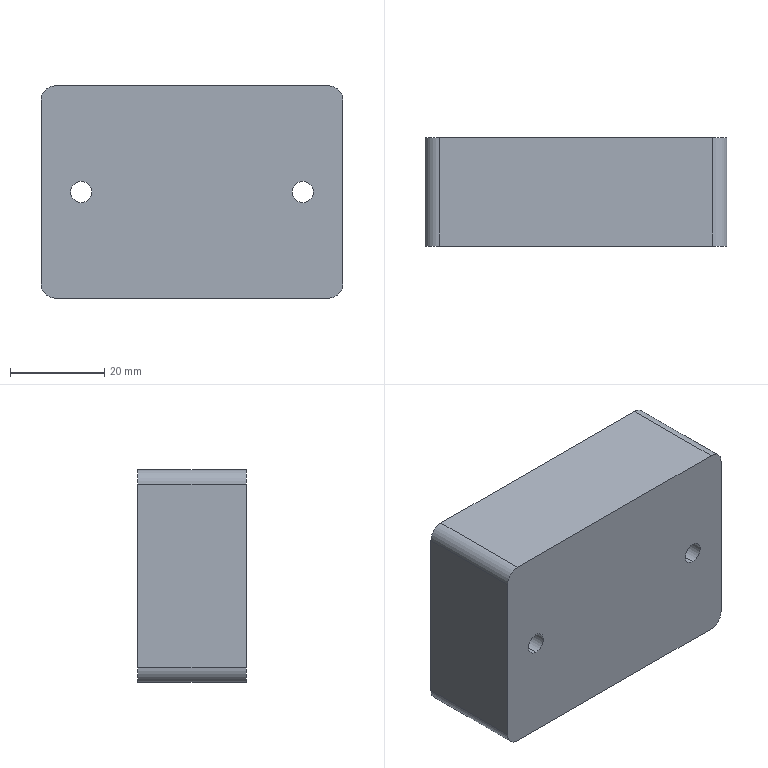Part | SolidWorks | features Extrusion 1, Fillet 1, HoleWzd 1 | 1 solid | 20 faces | box 64 x 23 x 45 mm | volume 65028 mm3 | cylinder 12 | plane 8 | commonest cylinder face diameters 4.5 x4 6 x4 8 x4
STEP:
#1=CARTESIAN_POINT('',(-23.5,7.1,-4.));
#2=VERTEX_POINT('',#1);
#3=CARTESIAN_POINT('',(-23.5,7.1,4.));
#4=VERTEX_POINT('',#3);
#5=CARTESIAN_POINT('',(-23.5,7.1,0.));
#6=DIRECTION('',(0.,1.,0.));
#7=DIRECTION('',(0.,0.,1.));
#8=AXIS2_PLACEMENT_3D('',#5,#6,#7);
#9=CIRCLE('',#8,4.);
#10=EDGE_CURVE('',#2,#4,#9,.T.);
#11=ORIENTED_EDGE('',*,*,#10,.F.);
#12=CARTESIAN_POINT('',(-23.5,11.5,-4.));
#13=VERTEX_POINT('',#12);
#14=CARTESIAN_POINT('',(-23.5,11.5,-4.));
#15=DIRECTION('',(0.,1.,0.));
#16=VECTOR('',#15,1000.);
#17=LINE('',#14,#16);
#18=EDGE_CURVE('',#2,#13,#17,.T.);
#19=ORIENTED_EDGE('',*,*,#18,.T.);
#20=CARTESIAN_POINT('',(-23.5,11.5,4.));
#21=VERTEX_POINT('',#20);
#22=CARTESIAN_POINT('',(-23.5,11.5,0.));
#23=DIRECTION('',(0.,1.,0.));
#24=DIRECTION('',(0.,0.,1.));
#25=AXIS2_PLACEMENT_3D('',#22,#23,#24);
#26=CIRCLE('',#25,4.);
#27=EDGE_CURVE('',#13,#21,#26,.T.);
#28=ORIENTED_EDGE('',*,*,#27,.T.);
#29=CARTESIAN_POINT('',(-23.5,11.5,4.));
#30=DIRECTION('',(0.,1.,0.));
#31=VECTOR('',#30,1000.);
#32=LINE('',#29,#31);
#33=EDGE_CURVE('',#4,#21,#32,.T.);
#34=ORIENTED_EDGE('',*,*,#33,.F.);
#35=EDGE_LOOP('',(#11,#19,#28,#34));
#36=FACE_OUTER_BOUND('',#35,.T.);
#37=CARTESIAN_POINT('',(-23.5,11.5,0.));
#38=DIRECTION('',(0.,1.,0.));
#39=DIRECTION('',(0.,0.,1.));
#40=AXIS2_PLACEMENT_3D('',#37,#38,#39);
#41=CYLINDRICAL_SURFACE('',#40,4.);
#42=ADVANCED_FACE('',(#36),#41,.F.);
#43=CARTESIAN_POINT('',(-23.5,-11.5,-2.25));
#44=VERTEX_POINT('',#43);
#45=CARTESIAN_POINT('',(-23.5,-11.5,2.25));
#46=VERTEX_POINT('',#45);
#47=CARTESIAN_POINT('',(-23.5,-11.5,0.));
#48=DIRECTION('',(0.,1.,0.));
#49=DIRECTION('',(0.,0.,1.));
#50=AXIS2_PLACEMENT_3D('',#47,#48,#49);
#51=CIRCLE('',#50,2.25);
#52=EDGE_CURVE('',#44,#46,#51,.T.);
#53=ORIENTED_EDGE('',*,*,#52,.F.);
#54=CARTESIAN_POINT('',(-23.5,7.1,-2.25));
#55=VERTEX_POINT('',#54);
#56=CARTESIAN_POINT('',(-23.5,11.5,-2.25));
#57=DIRECTION('',(0.,1.,0.));
#58=VECTOR('',#57,1000.);
#59=LINE('',#56,#58);
#60=EDGE_CURVE('',#44,#55,#59,.T.);
#61=ORIENTED_EDGE('',*,*,#60,.T.);
#62=CARTESIAN_POINT('',(-23.5,7.1,2.25));
#63=VERTEX_POINT('',#62);
#64=CARTESIAN_POINT('',(-23.5,7.1,0.));
#65=DIRECTION('',(0.,1.,0.));
#66=DIRECTION('',(0.,0.,1.));
#67=AXIS2_PLACEMENT_3D('',#64,#65,#66);
#68=CIRCLE('',#67,2.25);
#69=EDGE_CURVE('',#55,#63,#68,.T.);
#70=ORIENTED_EDGE('',*,*,#69,.T.);
#71=CARTESIAN_POINT('',(-23.5,11.5,2.25));
#72=DIRECTION('',(0.,1.,0.));
#73=VECTOR('',#72,1000.);
#74=LINE('',#71,#73);
#75=EDGE_CURVE('',#46,#63,#74,.T.);
#76=ORIENTED_EDGE('',*,*,#75,.F.);
#77=EDGE_LOOP('',(#53,#61,#70,#76));
#78=FACE_OUTER_BOUND('',#77,.T.);
#79=CARTESIAN_POINT('',(-23.5,11.5,0.));
#80=DIRECTION('',(0.,1.,0.));
#81=DIRECTION('',(0.,0.,1.));
#82=AXIS2_PLACEMENT_3D('',#79,#80,#81);
#83=CYLINDRICAL_SURFACE('',#82,2.25);
#84=ADVANCED_FACE('',(#78),#83,.F.);
#85=CARTESIAN_POINT('',(23.5,7.1,-4.));
#86=VERTEX_POINT('',#85);
#87=CARTESIAN_POINT('',(23.5,7.1,4.));
#88=VERTEX_POINT('',#87);
#89=CARTESIAN_POINT('',(23.5,7.1,0.));
#90=DIRECTION('',(0.,1.,0.));
#91=DIRECTION('',(0.,0.,1.));
#92=AXIS2_PLACEMENT_3D('',#89,#90,#91);
#93=CIRCLE('',#92,4.);
#94=EDGE_CURVE('',#86,#88,#93,.T.);
#95=ORIENTED_EDGE('',*,*,#94,.F.);
#96=CARTESIAN_POINT('',(23.5,11.5,-4.));
#97=VERTEX_POINT('',#96);
#98=CARTESIAN_POINT('',(23.5,11.5,-4.));
#99=DIRECTION('',(0.,1.,0.));
#100=VECTOR('',#99,1000.);
#101=LINE('',#98,#100);
#102=EDGE_CURVE('',#86,#97,#101,.T.);
#103=ORIENTED_EDGE('',*,*,#102,.T.);
#104=CARTESIAN_POINT('',(23.5,11.5,4.));
#105=VERTEX_POINT('',#104);
#106=CARTESIAN_POINT('',(23.5,11.5,0.));
#107=DIRECTION('',(0.,1.,0.));
#108=DIRECTION('',(0.,0.,1.));
#109=AXIS2_PLACEMENT_3D('',#106,#107,#108);
#110=CIRCLE('',#109,4.);
#111=EDGE_CURVE('',#97,#105,#110,.T.);
#112=ORIENTED_EDGE('',*,*,#111,.T.);
#113=CARTESIAN_POINT('',(23.5,11.5,4.));
#114=DIRECTION('',(0.,1.,0.));
#115=VECTOR('',#114,1000.);
#116=LINE('',#113,#115);
#117=EDGE_CURVE('',#88,#105,#116,.T.);
#118=ORIENTED_EDGE('',*,*,#117,.F.);
#119=EDGE_LOOP('',(#95,#103,#112,#118));
#120=FACE_OUTER_BOUND('',#119,.T.);
#121=CARTESIAN_POINT('',(23.5,11.5,0.));
#122=DIRECTION('',(0.,1.,0.));
#123=DIRECTION('',(0.,0.,1.));
#124=AXIS2_PLACEMENT_3D('',#121,#122,#123);
#125=CYLINDRICAL_SURFACE('',#124,4.);
#126=ADVANCED_FACE('',(#120),#125,.F.);
#127=CARTESIAN_POINT('',(23.5,-11.5,-2.25));
#128=VERTEX_POINT('',#127);
#129=CARTESIAN_POINT('',(23.5,-11.5,2.25));
#130=VERTEX_POINT('',#129);
#131=CARTESIAN_POINT('',(23.5,-11.5,0.));
#132=DIRECTION('',(0.,1.,0.));
#133=DIRECTION('',(0.,0.,1.));
#134=AXIS2_PLACEMENT_3D('',#131,#132,#133);
#135=CIRCLE('',#134,2.25);
#136=EDGE_CURVE('',#128,#130,#135,.T.);
#137=ORIENTED_EDGE('',*,*,#136,.F.);
#138=CARTESIAN_POINT('',(23.5,7.1,-2.25));
#139=VERTEX_POINT('',#138);
#140=CARTESIAN_POINT('',(23.5,11.5,-2.25));
#141=DIRECTION('',(0.,1.,0.));
#142=VECTOR('',#141,1000.);
#143=LINE('',#140,#142);
#144=EDGE_CURVE('',#128,#139,#143,.T.);
#145=ORIENTED_EDGE('',*,*,#144,.T.);
#146=CARTESIAN_POINT('',(23.5,7.1,2.25));
#147=VERTEX_POINT('',#146);
#148=CARTESIAN_POINT('',(23.5,7.1,0.));
#149=DIRECTION('',(0.,1.,0.));
#150=DIRECTION('',(0.,0.,1.));
#151=AXIS2_PLACEMENT_3D('',#148,#149,#150);
#152=CIRCLE('',#151,2.25);
#153=EDGE_CURVE('',#139,#147,#152,.T.);
#154=ORIENTED_EDGE('',*,*,#153,.T.);
#155=CARTESIAN_POINT('',(23.5,11.5,2.25));
#156=DIRECTION('',(0.,1.,0.));
#157=VECTOR('',#156,1000.);
#158=LINE('',#155,#157);
#159=EDGE_CURVE('',#130,#147,#158,.T.);
#160=ORIENTED_EDGE('',*,*,#159,.F.);
#161=EDGE_LOOP('',(#137,#145,#154,#160));
#162=FACE_OUTER_BOUND('',#161,.T.);
#163=CARTESIAN_POINT('',(23.5,11.5,0.));
#164=DIRECTION('',(0.,1.,0.));
#165=DIRECTION('',(0.,0.,1.));
#166=AXIS2_PLACEMENT_3D('',#163,#164,#165);
#167=CYLINDRICAL_SURFACE('',#166,2.25);
#168=ADVANCED_FACE('',(#162),#167,.F.);
#169=CARTESIAN_POINT('',(32.,11.5,19.5));
#170=VERTEX_POINT('',#169);
#171=CARTESIAN_POINT('',(32.,11.5,-19.5));
#172=VERTEX_POINT('',#171);
#173=CARTESIAN_POINT('',(32.,11.5,22.5));
#174=DIRECTION('',(0.,0.,-1.));
#175=VECTOR('',#174,1000.);
#176=LINE('',#173,#175);
#177=EDGE_CURVE('',#170,#172,#176,.T.);
#178=ORIENTED_EDGE('',*,*,#177,.F.);
#179=CARTESIAN_POINT('',(32.,-11.5,19.5));
#180=VERTEX_POINT('',#179);
#181=CARTESIAN_POINT('',(32.,11.5,19.5));
#182=DIRECTION('',(0.,-1.,0.));
#183=VECTOR('',#182,1000.);
#184=LINE('',#181,#183);
#185=EDGE_CURVE('',#170,#180,#184,.T.);
#186=ORIENTED_EDGE('',*,*,#185,.T.);
#187=CARTESIAN_POINT('',(32.,-11.5,-19.5));
#188=VERTEX_POINT('',#187);
#189=CARTESIAN_POINT('',(32.,-11.5,22.5));
#190=DIRECTION('',(0.,0.,-1.));
#191=VECTOR('',#190,1000.);
#192=LINE('',#189,#191);
#193=EDGE_CURVE('',#180,#188,#192,.T.);
#194=ORIENTED_EDGE('',*,*,#193,.T.);
#195=CARTESIAN_POINT('',(32.,11.5,-19.5));
#196=DIRECTION('',(0.,1.,0.));
#197=VECTOR('',#196,1000.);
#198=LINE('',#195,#197);
#199=EDGE_CURVE('',#188,#172,#198,.T.);
#200=ORIENTED_EDGE('',*,*,#199,.T.);
#201=EDGE_LOOP('',(#178,#186,#194,#200));
#202=FACE_OUTER_BOUND('',#201,.T.);
#203=CARTESIAN_POINT('',(32.,11.5,22.5));
#204=DIRECTION('',(-1.,0.,0.));
#205=DIRECTION('',(0.,0.,1.));
#206=AXIS2_PLACEMENT_3D('',#203,#204,#205);
#207=PLANE('',#206);
#208=ADVANCED_FACE('',(#202),#207,.F.);
#209=CARTESIAN_POINT('',(29.,11.5,-22.5));
#210=VERTEX_POINT('',#209);
#211=CARTESIAN_POINT('',(-29.,11.5,-22.5));
#212=VERTEX_POINT('',#211);
#213=CARTESIAN_POINT('',(-32.,11.5,-22.5));
#214=DIRECTION('',(-1.,0.,0.));
#215=VECTOR('',#214,1000.);
#216=LINE('',#213,#215);
#217=EDGE_CURVE('',#210,#212,#216,.T.);
#218=ORIENTED_EDGE('',*,*,#217,.F.);
#219=CARTESIAN_POINT('',(29.,-11.5,-22.5));
#220=VERTEX_POINT('',#219);
#221=CARTESIAN_POINT('',(29.,11.5,-22.5));
#222=DIRECTION('',(0.,-1.,0.));
#223=VECTOR('',#222,1000.);
#224=LINE('',#221,#223);
#225=EDGE_CURVE('',#210,#220,#224,.T.);
#226=ORIENTED_EDGE('',*,*,#225,.T.);
#227=CARTESIAN_POINT('',(-29.,-11.5,-22.5));
#228=VERTEX_POINT('',#227);
#229=CARTESIAN_POINT('',(-32.,-11.5,-22.5));
#230=DIRECTION('',(-1.,0.,0.));
#231=VECTOR('',#230,1000.);
#232=LINE('',#229,#231);
#233=EDGE_CURVE('',#220,#228,#232,.T.);
#234=ORIENTED_EDGE('',*,*,#233,.T.);
#235=CARTESIAN_POINT('',(-29.,11.5,-22.5));
#236=DIRECTION('',(0.,1.,0.));
#237=VECTOR('',#236,1000.);
#238=LINE('',#235,#237);
#239=EDGE_CURVE('',#228,#212,#238,.T.);
#240=ORIENTED_EDGE('',*,*,#239,.T.);
#241=EDGE_LOOP('',(#218,#226,#234,#240));
#242=FACE_OUTER_BOUND('',#241,.T.);
#243=CARTESIAN_POINT('',(-32.,11.5,-22.5));
#244=DIRECTION('',(0.,0.,1.));
#245=DIRECTION('',(1.,0.,0.));
#246=AXIS2_PLACEMENT_3D('',#243,#244,#245);
#247=PLANE('',#246);
#248=ADVANCED_FACE('',(#242),#247,.F.);
#249=CARTESIAN_POINT('',(-32.,11.5,-19.5));
#250=VERTEX_POINT('',#249);
#251=CARTESIAN_POINT('',(-32.,11.5,19.5));
#252=VERTEX_POINT('',#251);
#253=CARTESIAN_POINT('',(-32.,11.5,22.5));
#254=DIRECTION('',(0.,0.,1.));
#255=VECTOR('',#254,1000.);
#256=LINE('',#253,#255);
#257=EDGE_CURVE('',#250,#252,#256,.T.);
#258=ORIENTED_EDGE('',*,*,#257,.F.);
#259=CARTESIAN_POINT('',(-32.,-11.5,-19.5));
#260=VERTEX_POINT('',#259);
#261=CARTESIAN_POINT('',(-32.,11.5,-19.5));
#262=DIRECTION('',(0.,-1.,0.));
#263=VECTOR('',#262,1000.);
#264=LINE('',#261,#263);
#265=EDGE_CURVE('',#250,#260,#264,.T.);
#266=ORIENTED_EDGE('',*,*,#265,.T.);
#267=CARTESIAN_POINT('',(-32.,-11.5,19.5));
#268=VERTEX_POINT('',#267);
#269=CARTESIAN_POINT('',(-32.,-11.5,22.5));
#270=DIRECTION('',(0.,0.,1.));
#271=VECTOR('',#270,1000.);
#272=LINE('',#269,#271);
#273=EDGE_CURVE('',#260,#268,#272,.T.);
#274=ORIENTED_EDGE('',*,*,#273,.T.);
#275=CARTESIAN_POINT('',(-32.,11.5,19.5));
#276=DIRECTION('',(0.,1.,0.));
#277=VECTOR('',#276,1000.);
#278=LINE('',#275,#277);
#279=EDGE_CURVE('',#268,#252,#278,.T.);
#280=ORIENTED_EDGE('',*,*,#279,.T.);
#281=EDGE_LOOP('',(#258,#266,#274,#280));
#282=FACE_OUTER_BOUND('',#281,.T.);
#283=CARTESIAN_POINT('',(-32.,11.5,22.5));
#284=DIRECTION('',(1.,0.,0.));
#285=DIRECTION('',(0.,0.,-1.));
#286=AXIS2_PLACEMENT_3D('',#283,#284,#285);
#287=PLANE('',#286);
#288=ADVANCED_FACE('',(#282),#287,.F.);
#289=CARTESIAN_POINT('',(-29.,-11.5,22.5));
#290=VERTEX_POINT('',#289);
#291=CARTESIAN_POINT('',(29.,-11.5,22.5));
#292=VERTEX_POINT('',#291);
#293=CARTESIAN_POINT('',(-32.,-11.5,22.5));
#294=DIRECTION('',(1.,0.,0.));
#295=VECTOR('',#294,1000.);
#296=LINE('',#293,#295);
#297=EDGE_CURVE('',#290,#292,#296,.T.);
#298=ORIENTED_EDGE('',*,*,#297,.T.);
#299=CARTESIAN_POINT('',(29.,11.5,22.5));
#300=VERTEX_POINT('',#299);
#301=CARTESIAN_POINT('',(29.,11.5,22.5));
#302=DIRECTION('',(0.,1.,0.));
#303=VECTOR('',#302,1000.);
#304=LINE('',#301,#303);
#305=EDGE_CURVE('',#292,#300,#304,.T.);
#306=ORIENTED_EDGE('',*,*,#305,.T.);
#307=CARTESIAN_POINT('',(-29.,11.5,22.5));
#308=VERTEX_POINT('',#307);
#309=CARTESIAN_POINT('',(-32.,11.5,22.5));
#310=DIRECTION('',(1.,0.,0.));
#311=VECTOR('',#310,1000.);
#312=LINE('',#309,#311);
#313=EDGE_CURVE('',#308,#300,#312,.T.);
#314=ORIENTED_EDGE('',*,*,#313,.F.);
#315=CARTESIAN_POINT('',(-29.,11.5,22.5));
#316=DIRECTION('',(0.,-1.,0.));
#317=VECTOR('',#316,1000.);
#318=LINE('',#315,#317);
#319=EDGE_CURVE('',#308,#290,#318,.T.);
#320=ORIENTED_EDGE('',*,*,#319,.T.);
#321=EDGE_LOOP('',(#298,#306,#314,#320));
#322=FACE_OUTER_BOUND('',#321,.T.);
#323=CARTESIAN_POINT('',(-32.,11.5,22.5));
#324=DIRECTION('',(0.,0.,-1.));
#325=DIRECTION('',(-1.,0.,0.));
#326=AXIS2_PLACEMENT_3D('',#323,#324,#325);
#327=PLANE('',#326);
#328=ADVANCED_FACE('',(#322),#327,.F.);
#329=CARTESIAN_POINT('',(-23.5,11.5,0.));
#330=DIRECTION('',(0.,1.,0.));
#331=DIRECTION('',(0.,0.,1.));
#332=AXIS2_PLACEMENT_3D('',#329,#330,#331);
#333=CIRCLE('',#332,4.);
#334=EDGE_CURVE('',#21,#13,#333,.T.);
#335=ORIENTED_EDGE('',*,*,#334,.F.);
#336=ORIENTED_EDGE('',*,*,#27,.F.);
#337=EDGE_LOOP('',(#335,#336));
#338=FACE_BOUND('',#337,.T.);
#339=CARTESIAN_POINT('',(23.5,11.5,0.));
#340=DIRECTION('',(0.,1.,0.));
#341=DIRECTION('',(0.,0.,1.));
#342=AXIS2_PLACEMENT_3D('',#339,#340,#341);
#343=CIRCLE('',#342,4.);
#344=EDGE_CURVE('',#105,#97,#343,.T.);
#345=ORIENTED_EDGE('',*,*,#344,.F.);
#346=ORIENTED_EDGE('',*,*,#111,.F.);
#347=EDGE_LOOP('',(#345,#346));
#348=FACE_BOUND('',#347,.T.);
#349=ORIENTED_EDGE('',*,*,#313,.T.);
#350=CARTESIAN_POINT('',(29.,11.5,19.5));
#351=DIRECTION('',(0.,1.,0.));
#352=DIRECTION('',(0.,0.,-1.));
#353=AXIS2_PLACEMENT_3D('',#350,#351,#352);
#354=CIRCLE('',#353,3.);
#355=EDGE_CURVE('',#300,#170,#354,.T.);
#356=ORIENTED_EDGE('',*,*,#355,.T.);
#357=ORIENTED_EDGE('',*,*,#177,.T.);
#358=CARTESIAN_POINT('',(29.,11.5,-19.5));
#359=DIRECTION('',(0.,1.,0.));
#360=DIRECTION('',(0.,0.,-1.));
#361=AXIS2_PLACEMENT_3D('',#358,#359,#360);
#362=CIRCLE('',#361,3.);
#363=EDGE_CURVE('',#172,#210,#362,.T.);
#364=ORIENTED_EDGE('',*,*,#363,.T.);
#365=ORIENTED_EDGE('',*,*,#217,.T.);
#366=CARTESIAN_POINT('',(-29.,11.5,-19.5));
#367=DIRECTION('',(0.,1.,0.));
#368=DIRECTION('',(0.,0.,-1.));
#369=AXIS2_PLACEMENT_3D('',#366,#367,#368);
#370=CIRCLE('',#369,3.);
#371=EDGE_CURVE('',#212,#250,#370,.T.);
#372=ORIENTED_EDGE('',*,*,#371,.T.);
#373=ORIENTED_EDGE('',*,*,#257,.T.);
#374=CARTESIAN_POINT('',(-29.,11.5,19.5));
#375=DIRECTION('',(0.,1.,0.));
#376=DIRECTION('',(0.,0.,-1.));
#377=AXIS2_PLACEMENT_3D('',#374,#375,#376);
#378=CIRCLE('',#377,3.);
#379=EDGE_CURVE('',#252,#308,#378,.T.);
#380=ORIENTED_EDGE('',*,*,#379,.T.);
#381=EDGE_LOOP('',(#349,#356,#357,#364,#365,#372,#373,#380));
#382=FACE_OUTER_BOUND('',#381,.T.);
#383=CARTESIAN_POINT('',(0.,11.5,0.));
#384=DIRECTION('',(0.,-1.,0.));
#385=DIRECTION('',(0.,0.,-1.));
#386=AXIS2_PLACEMENT_3D('',#383,#384,#385);
#387=PLANE('',#386);
#388=ADVANCED_FACE('',(#338,#348,#382),#387,.F.);
#389=CARTESIAN_POINT('',(-23.5,-11.5,0.));
#390=DIRECTION('',(0.,1.,0.));
#391=DIRECTION('',(0.,0.,1.));
#392=AXIS2_PLACEMENT_3D('',#389,#390,#391);
#393=CIRCLE('',#392,2.25);
#394=EDGE_CURVE('',#46,#44,#393,.T.);
#395=ORIENTED_EDGE('',*,*,#394,.T.);
#396=ORIENTED_EDGE('',*,*,#52,.T.);
#397=EDGE_LOOP('',(#395,#396));
#398=FACE_BOUND('',#397,.T.);
#399=CARTESIAN_POINT('',(23.5,-11.5,0.));
#400=DIRECTION('',(0.,1.,0.));
#401=DIRECTION('',(0.,0.,1.));
#402=AXIS2_PLACEMENT_3D('',#399,#400,#401);
#403=CIRCLE('',#402,2.25);
#404=EDGE_CURVE('',#130,#128,#403,.T.);
#405=ORIENTED_EDGE('',*,*,#404,.T.);
#406=ORIENTED_EDGE('',*,*,#136,.T.);
#407=EDGE_LOOP('',(#405,#406));
#408=FACE_BOUND('',#407,.T.);
#409=ORIENTED_EDGE('',*,*,#193,.F.);
#410=CARTESIAN_POINT('',(29.,-11.5,19.5));
#411=DIRECTION('',(0.,-1.,0.));
#412=DIRECTION('',(0.,0.,-1.));
#413=AXIS2_PLACEMENT_3D('',#410,#411,#412);
#414=CIRCLE('',#413,3.);
#415=EDGE_CURVE('',#180,#292,#414,.T.);
#416=ORIENTED_EDGE('',*,*,#415,.T.);
#417=ORIENTED_EDGE('',*,*,#297,.F.);
#418=CARTESIAN_POINT('',(-29.,-11.5,19.5));
#419=DIRECTION('',(0.,-1.,0.));
#420=DIRECTION('',(0.,0.,-1.));
#421=AXIS2_PLACEMENT_3D('',#418,#419,#420);
#422=CIRCLE('',#421,3.);
#423=EDGE_CURVE('',#290,#268,#422,.T.);
#424=ORIENTED_EDGE('',*,*,#423,.T.);
#425=ORIENTED_EDGE('',*,*,#273,.F.);
#426=CARTESIAN_POINT('',(-29.,-11.5,-19.5));
#427=DIRECTION('',(0.,-1.,0.));
#428=DIRECTION('',(0.,0.,-1.));
#429=AXIS2_PLACEMENT_3D('',#426,#427,#428);
#430=CIRCLE('',#429,3.);
#431=EDGE_CURVE('',#260,#228,#430,.T.);
#432=ORIENTED_EDGE('',*,*,#431,.T.);
#433=ORIENTED_EDGE('',*,*,#233,.F.);
#434=CARTESIAN_POINT('',(29.,-11.5,-19.5));
#435=DIRECTION('',(0.,-1.,0.));
#436=DIRECTION('',(0.,0.,-1.));
#437=AXIS2_PLACEMENT_3D('',#434,#435,#436);
#438=CIRCLE('',#437,3.);
#439=EDGE_CURVE('',#220,#188,#438,.T.);
#440=ORIENTED_EDGE('',*,*,#439,.T.);
#441=EDGE_LOOP('',(#409,#416,#417,#424,#425,#432,#433,#440));
#442=FACE_OUTER_BOUND('',#441,.T.);
#443=CARTESIAN_POINT('',(0.,-11.5,0.));
#444=DIRECTION('',(0.,-1.,0.));
#445=DIRECTION('',(0.,0.,-1.));
#446=AXIS2_PLACEMENT_3D('',#443,#444,#445);
#447=PLANE('',#446);
#448=ADVANCED_FACE('',(#398,#408,#442),#447,.T.);
#449=ORIENTED_EDGE('',*,*,#144,.F.);
#450=ORIENTED_EDGE('',*,*,#404,.F.);
#451=ORIENTED_EDGE('',*,*,#159,.T.);
#452=CARTESIAN_POINT('',(23.5,7.1,0.));
#453=DIRECTION('',(0.,1.,0.));
#454=DIRECTION('',(0.,0.,1.));
#455=AXIS2_PLACEMENT_3D('',#452,#453,#454);
#456=CIRCLE('',#455,2.25);
#457=EDGE_CURVE('',#147,#139,#456,.T.);
#458=ORIENTED_EDGE('',*,*,#457,.T.);
#459=EDGE_LOOP('',(#449,#450,#451,#458));
#460=FACE_OUTER_BOUND('',#459,.T.);
#461=CARTESIAN_POINT('',(23.5,11.5,0.));
#462=DIRECTION('',(0.,1.,0.));
#463=DIRECTION('',(0.,0.,1.));
#464=AXIS2_PLACEMENT_3D('',#461,#462,#463);
#465=CYLINDRICAL_SURFACE('',#464,2.25);
#466=ADVANCED_FACE('',(#460),#465,.F.);
#467=ORIENTED_EDGE('',*,*,#457,.F.);
#468=ORIENTED_EDGE('',*,*,#153,.F.);
#469=EDGE_LOOP('',(#467,#468));
#470=FACE_BOUND('',#469,.T.);
#471=CARTESIAN_POINT('',(23.5,7.1,0.));
#472=DIRECTION('',(0.,1.,0.));
#473=DIRECTION('',(0.,0.,1.));
#474=AXIS2_PLACEMENT_3D('',#471,#472,#473);
#475=CIRCLE('',#474,4.);
#476=EDGE_CURVE('',#88,#86,#475,.T.);
#477=ORIENTED_EDGE('',*,*,#476,.T.);
#478=ORIENTED_EDGE('',*,*,#94,.T.);
#479=EDGE_LOOP('',(#477,#478));
#480=FACE_OUTER_BOUND('',#479,.T.);
#481=CARTESIAN_POINT('',(25.75,7.1,0.));
#482=DIRECTION('',(0.,-1.,0.));
#483=DIRECTION('',(0.,0.,-1.));
#484=AXIS2_PLACEMENT_3D('',#481,#482,#483);
#485=PLANE('',#484);
#486=ADVANCED_FACE('',(#470,#480),#485,.F.);
#487=ORIENTED_EDGE('',*,*,#102,.F.);
#488=ORIENTED_EDGE('',*,*,#476,.F.);
#489=ORIENTED_EDGE('',*,*,#117,.T.);
#490=ORIENTED_EDGE('',*,*,#344,.T.);
#491=EDGE_LOOP('',(#487,#488,#489,#490));
#492=FACE_OUTER_BOUND('',#491,.T.);
#493=CARTESIAN_POINT('',(23.5,11.5,0.));
#494=DIRECTION('',(0.,1.,0.));
#495=DIRECTION('',(0.,0.,1.));
#496=AXIS2_PLACEMENT_3D('',#493,#494,#495);
#497=CYLINDRICAL_SURFACE('',#496,4.);
#498=ADVANCED_FACE('',(#492),#497,.F.);
#499=ORIENTED_EDGE('',*,*,#60,.F.);
#500=ORIENTED_EDGE('',*,*,#394,.F.);
#501=ORIENTED_EDGE('',*,*,#75,.T.);
#502=CARTESIAN_POINT('',(-23.5,7.1,0.));
#503=DIRECTION('',(0.,1.,0.));
#504=DIRECTION('',(0.,0.,1.));
#505=AXIS2_PLACEMENT_3D('',#502,#503,#504);
#506=CIRCLE('',#505,2.25);
#507=EDGE_CURVE('',#63,#55,#506,.T.);
#508=ORIENTED_EDGE('',*,*,#507,.T.);
#509=EDGE_LOOP('',(#499,#500,#501,#508));
#510=FACE_OUTER_BOUND('',#509,.T.);
#511=CARTESIAN_POINT('',(-23.5,11.5,0.));
#512=DIRECTION('',(0.,1.,0.));
#513=DIRECTION('',(0.,0.,1.));
#514=AXIS2_PLACEMENT_3D('',#511,#512,#513);
#515=CYLINDRICAL_SURFACE('',#514,2.25);
#516=ADVANCED_FACE('',(#510),#515,.F.);
#517=ORIENTED_EDGE('',*,*,#507,.F.);
#518=ORIENTED_EDGE('',*,*,#69,.F.);
#519=EDGE_LOOP('',(#517,#518));
#520=FACE_BOUND('',#519,.T.);
#521=CARTESIAN_POINT('',(-23.5,7.1,0.));
#522=DIRECTION('',(0.,1.,0.));
#523=DIRECTION('',(0.,0.,1.));
#524=AXIS2_PLACEMENT_3D('',#521,#522,#523);
#525=CIRCLE('',#524,4.);
#526=EDGE_CURVE('',#4,#2,#525,.T.);
#527=ORIENTED_EDGE('',*,*,#526,.T.);
#528=ORIENTED_EDGE('',*,*,#10,.T.);
#529=EDGE_LOOP('',(#527,#528));
#530=FACE_OUTER_BOUND('',#529,.T.);
#531=CARTESIAN_POINT('',(-21.25,7.1,0.));
#532=DIRECTION('',(0.,-1.,0.));
#533=DIRECTION('',(0.,0.,-1.));
#534=AXIS2_PLACEMENT_3D('',#531,#532,#533);
#535=PLANE('',#534);
#536=ADVANCED_FACE('',(#520,#530),#535,.F.);
#537=ORIENTED_EDGE('',*,*,#18,.F.);
#538=ORIENTED_EDGE('',*,*,#526,.F.);
#539=ORIENTED_EDGE('',*,*,#33,.T.);
#540=ORIENTED_EDGE('',*,*,#334,.T.);
#541=EDGE_LOOP('',(#537,#538,#539,#540));
#542=FACE_OUTER_BOUND('',#541,.T.);
#543=CARTESIAN_POINT('',(-23.5,11.5,0.));
#544=DIRECTION('',(0.,1.,0.));
#545=DIRECTION('',(0.,0.,1.));
#546=AXIS2_PLACEMENT_3D('',#543,#544,#545);
#547=CYLINDRICAL_SURFACE('',#546,4.);
#548=ADVANCED_FACE('',(#542),#547,.F.);
#549=ORIENTED_EDGE('',*,*,#355,.F.);
#550=ORIENTED_EDGE('',*,*,#305,.F.);
#551=ORIENTED_EDGE('',*,*,#415,.F.);
#552=ORIENTED_EDGE('',*,*,#185,.F.);
#553=EDGE_LOOP('',(#549,#550,#551,#552));
#554=FACE_OUTER_BOUND('',#553,.T.);
#555=CARTESIAN_POINT('',(29.,11.5,19.5));
#556=DIRECTION('',(0.,-1.,0.));
#557=DIRECTION('',(0.,0.,-1.));
#558=AXIS2_PLACEMENT_3D('',#555,#556,#557);
#559=CYLINDRICAL_SURFACE('',#558,3.);
#560=ADVANCED_FACE('',(#554),#559,.T.);
#561=ORIENTED_EDGE('',*,*,#363,.F.);
#562=ORIENTED_EDGE('',*,*,#199,.F.);
#563=ORIENTED_EDGE('',*,*,#439,.F.);
#564=ORIENTED_EDGE('',*,*,#225,.F.);
#565=EDGE_LOOP('',(#561,#562,#563,#564));
#566=FACE_OUTER_BOUND('',#565,.T.);
#567=CARTESIAN_POINT('',(29.,11.5,-19.5));
#568=DIRECTION('',(0.,-1.,0.));
#569=DIRECTION('',(0.,0.,-1.));
#570=AXIS2_PLACEMENT_3D('',#567,#568,#569);
#571=CYLINDRICAL_SURFACE('',#570,3.);
#572=ADVANCED_FACE('',(#566),#571,.T.);
#573=ORIENTED_EDGE('',*,*,#371,.F.);
#574=ORIENTED_EDGE('',*,*,#239,.F.);
#575=ORIENTED_EDGE('',*,*,#431,.F.);
#576=ORIENTED_EDGE('',*,*,#265,.F.);
#577=EDGE_LOOP('',(#573,#574,#575,#576));
#578=FACE_OUTER_BOUND('',#577,.T.);
#579=CARTESIAN_POINT('',(-29.,11.5,-19.5));
#580=DIRECTION('',(0.,-1.,0.));
#581=DIRECTION('',(0.,0.,-1.));
#582=AXIS2_PLACEMENT_3D('',#579,#580,#581);
#583=CYLINDRICAL_SURFACE('',#582,3.);
#584=ADVANCED_FACE('',(#578),#583,.T.);
#585=ORIENTED_EDGE('',*,*,#379,.F.);
#586=ORIENTED_EDGE('',*,*,#279,.F.);
#587=ORIENTED_EDGE('',*,*,#423,.F.);
#588=ORIENTED_EDGE('',*,*,#319,.F.);
#589=EDGE_LOOP('',(#585,#586,#587,#588));
#590=FACE_OUTER_BOUND('',#589,.T.);
#591=CARTESIAN_POINT('',(-29.,11.5,19.5));
#592=DIRECTION('',(0.,-1.,0.));
#593=DIRECTION('',(0.,0.,-1.));
#594=AXIS2_PLACEMENT_3D('',#591,#592,#593);
#595=CYLINDRICAL_SURFACE('',#594,3.);
#596=ADVANCED_FACE('',(#590),#595,.T.);
#597=CLOSED_SHELL('',(#42,#84,#126,#168,#208,#248,#288,#328,#388,#448,#466,#486,#498,#516,#536,#548,#560,#572,#584,#596));
#598=MANIFOLD_SOLID_BREP('',#597);
#599=CARTESIAN_POINT('',(0.,0.,0.));
#600=DIRECTION('',(0.,0.,1.));
#601=DIRECTION('',(1.,0.,0.));
#602=AXIS2_PLACEMENT_3D('',#599,#600,#601);
#603=(LENGTH_UNIT()NAMED_UNIT(*)SI_UNIT(.MILLI.,.METRE.));
#604=UNCERTAINTY_MEASURE_WITH_UNIT(LENGTH_MEASURE(0.00001),#603,'','');
#605=(NAMED_UNIT(*)PLANE_ANGLE_UNIT()SI_UNIT($,.RADIAN.));
#606=(NAMED_UNIT(*)SI_UNIT($,.STERADIAN.)SOLID_ANGLE_UNIT());
#607=(GEOMETRIC_REPRESENTATION_CONTEXT(3)GLOBAL_UNCERTAINTY_ASSIGNED_CONTEXT((#604))GLOBAL_UNIT_ASSIGNED_CONTEXT((#603,#605,#606))REPRESENTATION_CONTEXT('',''));
#608=ADVANCED_BREP_SHAPE_REPRESENTATION('',(#598,#602),#607);